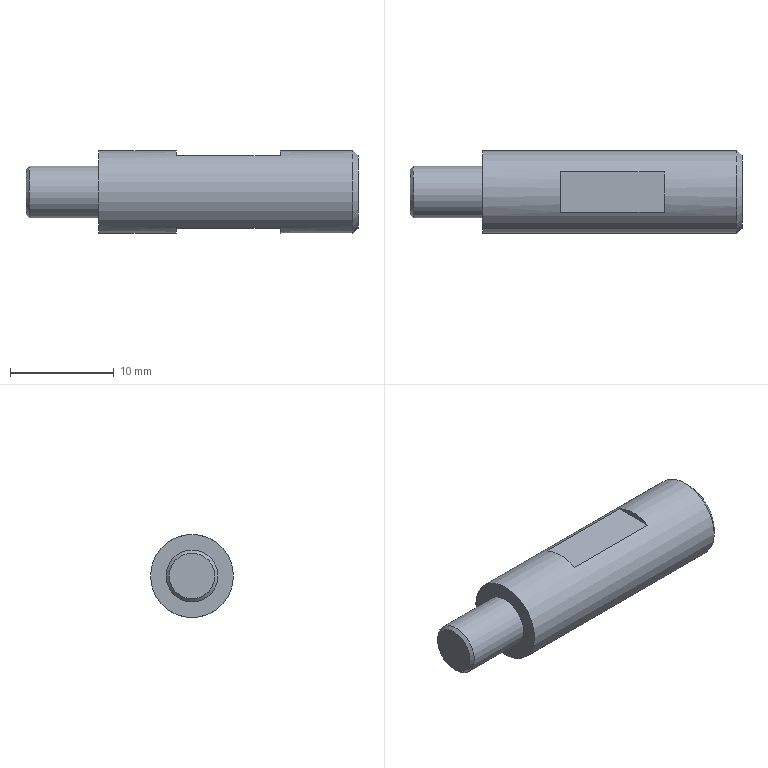Part | NX | features BREP 1 | 1 solid | 13 faces | box 32 x 8 x 8 mm | volume 1364 mm3 | plane 9 | cylinder 2 | cone 2 | commonest cylinder face diameters 5 x1 8 x1
STEP:
#1=CARTESIAN_POINT('',(-1.5,-1.936,3.5));
#2=VERTEX_POINT('',#1);
#3=CARTESIAN_POINT('',(8.5,-1.936,3.5));
#4=VERTEX_POINT('',#3);
#5=CARTESIAN_POINT('',(-16.,-1.936,3.5));
#6=DIRECTION('',(1.,0.,0.));
#7=VECTOR('',#6,1000.);
#8=LINE('',#5,#7);
#9=EDGE_CURVE('',#2,#4,#8,.T.);
#10=ORIENTED_EDGE('',*,*,#9,.F.);
#11=CARTESIAN_POINT('',(-1.5,1.936,3.5));
#12=VERTEX_POINT('',#11);
#13=CARTESIAN_POINT('',(-1.5,0.,0.));
#14=DIRECTION('',(-1.,0.,0.));
#15=DIRECTION('',(0.,0.,1.));
#16=AXIS2_PLACEMENT_3D('',#13,#14,#15);
#17=CIRCLE('',#16,4.);
#18=EDGE_CURVE('',#2,#12,#17,.T.);
#19=ORIENTED_EDGE('',*,*,#18,.T.);
#20=CARTESIAN_POINT('',(8.5,1.936,3.5));
#21=VERTEX_POINT('',#20);
#22=CARTESIAN_POINT('',(-16.,1.936,3.5));
#23=DIRECTION('',(-1.,0.,0.));
#24=VECTOR('',#23,1000.);
#25=LINE('',#22,#24);
#26=EDGE_CURVE('',#21,#12,#25,.T.);
#27=ORIENTED_EDGE('',*,*,#26,.F.);
#28=CARTESIAN_POINT('',(8.5,0.,0.));
#29=DIRECTION('',(-1.,0.,0.));
#30=DIRECTION('',(0.,0.,1.));
#31=AXIS2_PLACEMENT_3D('',#28,#29,#30);
#32=CIRCLE('',#31,4.);
#33=EDGE_CURVE('',#4,#21,#32,.T.);
#34=ORIENTED_EDGE('',*,*,#33,.F.);
#35=EDGE_LOOP('',(#10,#19,#27,#34));
#36=FACE_BOUND('',#35,.T.);
#37=CARTESIAN_POINT('',(-9.,-4.,0.));
#38=VERTEX_POINT('',#37);
#39=CARTESIAN_POINT('',(-9.,0.,0.));
#40=DIRECTION('',(1.,0.,0.));
#41=DIRECTION('',(0.,-1.,0.));
#42=AXIS2_PLACEMENT_3D('',#39,#40,#41);
#43=CIRCLE('',#42,4.);
#44=EDGE_CURVE('',#38,#38,#43,.T.);
#45=ORIENTED_EDGE('',*,*,#44,.T.);
#46=EDGE_LOOP('',(#45));
#47=FACE_BOUND('',#46,.T.);
#48=CARTESIAN_POINT('',(15.5,-4.,0.));
#49=VERTEX_POINT('',#48);
#50=CARTESIAN_POINT('',(15.5,0.,0.));
#51=DIRECTION('',(1.,0.,0.));
#52=DIRECTION('',(0.,-1.,0.));
#53=AXIS2_PLACEMENT_3D('',#50,#51,#52);
#54=CIRCLE('',#53,4.);
#55=EDGE_CURVE('',#49,#49,#54,.T.);
#56=ORIENTED_EDGE('',*,*,#55,.F.);
#57=EDGE_LOOP('',(#56));
#58=FACE_BOUND('',#57,.T.);
#59=CARTESIAN_POINT('',(8.5,-1.936,-3.5));
#60=VERTEX_POINT('',#59);
#61=CARTESIAN_POINT('',(8.5,1.936,-3.5));
#62=VERTEX_POINT('',#61);
#63=CARTESIAN_POINT('',(8.5,0.,0.));
#64=DIRECTION('',(1.,0.,0.));
#65=DIRECTION('',(0.,0.,-1.));
#66=AXIS2_PLACEMENT_3D('',#63,#64,#65);
#67=CIRCLE('',#66,4.);
#68=EDGE_CURVE('',#60,#62,#67,.T.);
#69=ORIENTED_EDGE('',*,*,#68,.T.);
#70=CARTESIAN_POINT('',(-1.5,1.936,-3.5));
#71=VERTEX_POINT('',#70);
#72=CARTESIAN_POINT('',(-16.,1.936,-3.5));
#73=DIRECTION('',(1.,0.,0.));
#74=VECTOR('',#73,1000.);
#75=LINE('',#72,#74);
#76=EDGE_CURVE('',#71,#62,#75,.T.);
#77=ORIENTED_EDGE('',*,*,#76,.F.);
#78=CARTESIAN_POINT('',(-1.5,-1.936,-3.5));
#79=VERTEX_POINT('',#78);
#80=CARTESIAN_POINT('',(-1.5,0.,0.));
#81=DIRECTION('',(1.,0.,0.));
#82=DIRECTION('',(0.,0.,-1.));
#83=AXIS2_PLACEMENT_3D('',#80,#81,#82);
#84=CIRCLE('',#83,4.);
#85=EDGE_CURVE('',#79,#71,#84,.T.);
#86=ORIENTED_EDGE('',*,*,#85,.F.);
#87=CARTESIAN_POINT('',(-16.,-1.936,-3.5));
#88=DIRECTION('',(-1.,0.,0.));
#89=VECTOR('',#88,1000.);
#90=LINE('',#87,#89);
#91=EDGE_CURVE('',#60,#79,#90,.T.);
#92=ORIENTED_EDGE('',*,*,#91,.F.);
#93=EDGE_LOOP('',(#69,#77,#86,#92));
#94=FACE_BOUND('',#93,.T.);
#95=CARTESIAN_POINT('',(-16.,0.,0.));
#96=DIRECTION('',(-1.,0.,0.));
#97=DIRECTION('',(0.,1.,0.));
#98=AXIS2_PLACEMENT_3D('',#95,#96,#97);
#99=CYLINDRICAL_SURFACE('',#98,4.);
#100=ADVANCED_FACE('',(#36,#47,#58,#94),#99,.T.);
#101=CARTESIAN_POINT('',(-16.,2.2,0.));
#102=VERTEX_POINT('',#101);
#103=CARTESIAN_POINT('',(-16.,0.,0.));
#104=DIRECTION('',(1.,0.,0.));
#105=DIRECTION('',(0.,1.,0.));
#106=AXIS2_PLACEMENT_3D('',#103,#104,#105);
#107=CIRCLE('',#106,2.2);
#108=EDGE_CURVE('',#102,#102,#107,.T.);
#109=ORIENTED_EDGE('',*,*,#108,.F.);
#110=EDGE_LOOP('',(#109));
#111=FACE_BOUND('',#110,.T.);
#112=CARTESIAN_POINT('',(-16.,0.,0.));
#113=DIRECTION('',(1.,0.,0.));
#114=DIRECTION('',(0.,-1.,0.));
#115=AXIS2_PLACEMENT_3D('',#112,#113,#114);
#116=PLANE('',#115);
#117=ADVANCED_FACE('',(#111),#116,.F.);
#118=CARTESIAN_POINT('',(-15.7,2.5,0.));
#119=VERTEX_POINT('',#118);
#120=CARTESIAN_POINT('',(-15.7,0.,0.));
#121=DIRECTION('',(-1.,0.,0.));
#122=DIRECTION('',(0.,1.,0.));
#123=AXIS2_PLACEMENT_3D('',#120,#121,#122);
#124=CIRCLE('',#123,2.5);
#125=EDGE_CURVE('',#119,#119,#124,.T.);
#126=ORIENTED_EDGE('',*,*,#125,.F.);
#127=EDGE_LOOP('',(#126));
#128=FACE_BOUND('',#127,.T.);
#129=CARTESIAN_POINT('',(-9.,-2.5,0.));
#130=VERTEX_POINT('',#129);
#131=CARTESIAN_POINT('',(-9.,0.,0.));
#132=DIRECTION('',(1.,0.,0.));
#133=DIRECTION('',(0.,-1.,0.));
#134=AXIS2_PLACEMENT_3D('',#131,#132,#133);
#135=CIRCLE('',#134,2.5);
#136=EDGE_CURVE('',#130,#130,#135,.T.);
#137=ORIENTED_EDGE('',*,*,#136,.F.);
#138=EDGE_LOOP('',(#137));
#139=FACE_BOUND('',#138,.T.);
#140=CARTESIAN_POINT('',(-16.,0.,0.));
#141=DIRECTION('',(-1.,0.,0.));
#142=DIRECTION('',(0.,1.,0.));
#143=AXIS2_PLACEMENT_3D('',#140,#141,#142);
#144=CYLINDRICAL_SURFACE('',#143,2.5);
#145=ADVANCED_FACE('',(#128,#139),#144,.T.);
#146=ORIENTED_EDGE('',*,*,#136,.T.);
#147=EDGE_LOOP('',(#146));
#148=FACE_BOUND('',#147,.T.);
#149=ORIENTED_EDGE('',*,*,#44,.F.);
#150=EDGE_LOOP('',(#149));
#151=FACE_BOUND('',#150,.T.);
#152=CARTESIAN_POINT('',(-9.,2.5,0.));
#153=DIRECTION('',(1.,0.,0.));
#154=DIRECTION('',(0.,-1.,0.));
#155=AXIS2_PLACEMENT_3D('',#152,#153,#154);
#156=PLANE('',#155);
#157=ADVANCED_FACE('',(#148,#151),#156,.F.);
#158=CARTESIAN_POINT('',(16.,-3.5,0.));
#159=VERTEX_POINT('',#158);
#160=CARTESIAN_POINT('',(16.,0.,0.));
#161=DIRECTION('',(-1.,0.,0.));
#162=DIRECTION('',(0.,-1.,0.));
#163=AXIS2_PLACEMENT_3D('',#160,#161,#162);
#164=CIRCLE('',#163,3.5);
#165=EDGE_CURVE('',#159,#159,#164,.T.);
#166=ORIENTED_EDGE('',*,*,#165,.F.);
#167=EDGE_LOOP('',(#166));
#168=FACE_BOUND('',#167,.T.);
#169=CARTESIAN_POINT('',(16.,0.,0.));
#170=DIRECTION('',(-1.,0.,0.));
#171=DIRECTION('',(0.,1.,0.));
#172=AXIS2_PLACEMENT_3D('',#169,#170,#171);
#173=PLANE('',#172);
#174=ADVANCED_FACE('',(#168),#173,.F.);
#175=ORIENTED_EDGE('',*,*,#165,.T.);
#176=EDGE_LOOP('',(#175));
#177=FACE_BOUND('',#176,.T.);
#178=ORIENTED_EDGE('',*,*,#55,.T.);
#179=EDGE_LOOP('',(#178));
#180=FACE_BOUND('',#179,.T.);
#181=CARTESIAN_POINT('',(15.5,0.,0.));
#182=DIRECTION('',(-1.,0.,0.));
#183=DIRECTION('',(0.,1.,0.));
#184=AXIS2_PLACEMENT_3D('',#181,#182,#183);
#185=CONICAL_SURFACE('',#184,4.,0.7854);
#186=ADVANCED_FACE('',(#177,#180),#185,.T.);
#187=ORIENTED_EDGE('',*,*,#125,.T.);
#188=EDGE_LOOP('',(#187));
#189=FACE_BOUND('',#188,.T.);
#190=ORIENTED_EDGE('',*,*,#108,.T.);
#191=EDGE_LOOP('',(#190));
#192=FACE_BOUND('',#191,.T.);
#193=CARTESIAN_POINT('',(-16.,0.,0.));
#194=DIRECTION('',(1.,0.,0.));
#195=DIRECTION('',(0.,-1.,0.));
#196=AXIS2_PLACEMENT_3D('',#193,#194,#195);
#197=CONICAL_SURFACE('',#196,2.2,0.7854);
#198=ADVANCED_FACE('',(#189,#192),#197,.T.);
#199=CARTESIAN_POINT('',(8.5,-3.194,-3.5));
#200=DIRECTION('',(0.,-1.,0.));
#201=VECTOR('',#200,1000.);
#202=LINE('',#199,#201);
#203=EDGE_CURVE('',#62,#60,#202,.T.);
#204=ORIENTED_EDGE('',*,*,#203,.T.);
#205=ORIENTED_EDGE('',*,*,#91,.T.);
#206=CARTESIAN_POINT('',(-1.5,-3.194,-3.5));
#207=DIRECTION('',(0.,-1.,0.));
#208=VECTOR('',#207,1000.);
#209=LINE('',#206,#208);
#210=EDGE_CURVE('',#71,#79,#209,.T.);
#211=ORIENTED_EDGE('',*,*,#210,.F.);
#212=ORIENTED_EDGE('',*,*,#76,.T.);
#213=EDGE_LOOP('',(#204,#205,#211,#212));
#214=FACE_BOUND('',#213,.T.);
#215=CARTESIAN_POINT('',(8.5,-3.194,-3.5));
#216=DIRECTION('',(0.,0.,1.));
#217=DIRECTION('',(0.,-1.,0.));
#218=AXIS2_PLACEMENT_3D('',#215,#216,#217);
#219=PLANE('',#218);
#220=ADVANCED_FACE('',(#214),#219,.F.);
#221=ORIENTED_EDGE('',*,*,#68,.F.);
#222=ORIENTED_EDGE('',*,*,#203,.F.);
#223=EDGE_LOOP('',(#221,#222));
#224=FACE_BOUND('',#223,.T.);
#225=CARTESIAN_POINT('',(8.5,0.,0.));
#226=DIRECTION('',(-1.,0.,0.));
#227=DIRECTION('',(0.,0.,1.));
#228=AXIS2_PLACEMENT_3D('',#225,#226,#227);
#229=PLANE('',#228);
#230=ADVANCED_FACE('',(#224),#229,.T.);
#231=ORIENTED_EDGE('',*,*,#210,.T.);
#232=ORIENTED_EDGE('',*,*,#85,.T.);
#233=EDGE_LOOP('',(#231,#232));
#234=FACE_BOUND('',#233,.T.);
#235=CARTESIAN_POINT('',(-1.5,0.,0.));
#236=DIRECTION('',(-1.,0.,0.));
#237=DIRECTION('',(0.,0.,1.));
#238=AXIS2_PLACEMENT_3D('',#235,#236,#237);
#239=PLANE('',#238);
#240=ADVANCED_FACE('',(#234),#239,.F.);
#241=CARTESIAN_POINT('',(8.5,-2.896,3.5));
#242=DIRECTION('',(0.,1.,0.));
#243=VECTOR('',#242,1000.);
#244=LINE('',#241,#243);
#245=EDGE_CURVE('',#4,#21,#244,.T.);
#246=ORIENTED_EDGE('',*,*,#245,.T.);
#247=ORIENTED_EDGE('',*,*,#26,.T.);
#248=CARTESIAN_POINT('',(-1.5,-2.896,3.5));
#249=DIRECTION('',(0.,1.,0.));
#250=VECTOR('',#249,1000.);
#251=LINE('',#248,#250);
#252=EDGE_CURVE('',#2,#12,#251,.T.);
#253=ORIENTED_EDGE('',*,*,#252,.F.);
#254=ORIENTED_EDGE('',*,*,#9,.T.);
#255=EDGE_LOOP('',(#246,#247,#253,#254));
#256=FACE_BOUND('',#255,.T.);
#257=CARTESIAN_POINT('',(8.5,-2.896,3.5));
#258=DIRECTION('',(0.,0.,-1.));
#259=DIRECTION('',(-1.,0.,0.));
#260=AXIS2_PLACEMENT_3D('',#257,#258,#259);
#261=PLANE('',#260);
#262=ADVANCED_FACE('',(#256),#261,.F.);
#263=ORIENTED_EDGE('',*,*,#245,.F.);
#264=ORIENTED_EDGE('',*,*,#33,.T.);
#265=EDGE_LOOP('',(#263,#264));
#266=FACE_BOUND('',#265,.T.);
#267=CARTESIAN_POINT('',(8.5,0.,0.));
#268=DIRECTION('',(1.,0.,0.));
#269=DIRECTION('',(0.,0.,-1.));
#270=AXIS2_PLACEMENT_3D('',#267,#268,#269);
#271=PLANE('',#270);
#272=ADVANCED_FACE('',(#266),#271,.F.);
#273=ORIENTED_EDGE('',*,*,#18,.F.);
#274=ORIENTED_EDGE('',*,*,#252,.T.);
#275=EDGE_LOOP('',(#273,#274));
#276=FACE_BOUND('',#275,.T.);
#277=CARTESIAN_POINT('',(-1.5,0.,0.));
#278=DIRECTION('',(1.,0.,0.));
#279=DIRECTION('',(0.,0.,-1.));
#280=AXIS2_PLACEMENT_3D('',#277,#278,#279);
#281=PLANE('',#280);
#282=ADVANCED_FACE('',(#276),#281,.T.);
#283=CLOSED_SHELL('',(#100,#117,#145,#157,#174,#186,#198,#220,#230,#240,#262,#272,#282));
#284=MANIFOLD_SOLID_BREP('',#283);
#285=(LENGTH_UNIT()NAMED_UNIT(*)SI_UNIT(.MILLI.,.METRE.));
#286=UNCERTAINTY_MEASURE_WITH_UNIT(LENGTH_MEASURE(0.00001),#285,'','');
#287=(NAMED_UNIT(*)PLANE_ANGLE_UNIT()SI_UNIT($,.RADIAN.));
#288=(NAMED_UNIT(*)SI_UNIT($,.STERADIAN.)SOLID_ANGLE_UNIT());
#289=(GEOMETRIC_REPRESENTATION_CONTEXT(3)GLOBAL_UNCERTAINTY_ASSIGNED_CONTEXT((#286))GLOBAL_UNIT_ASSIGNED_CONTEXT((#285,#287,#288))REPRESENTATION_CONTEXT('',''));
#290=ADVANCED_BREP_SHAPE_REPRESENTATION('',(#284),#289);